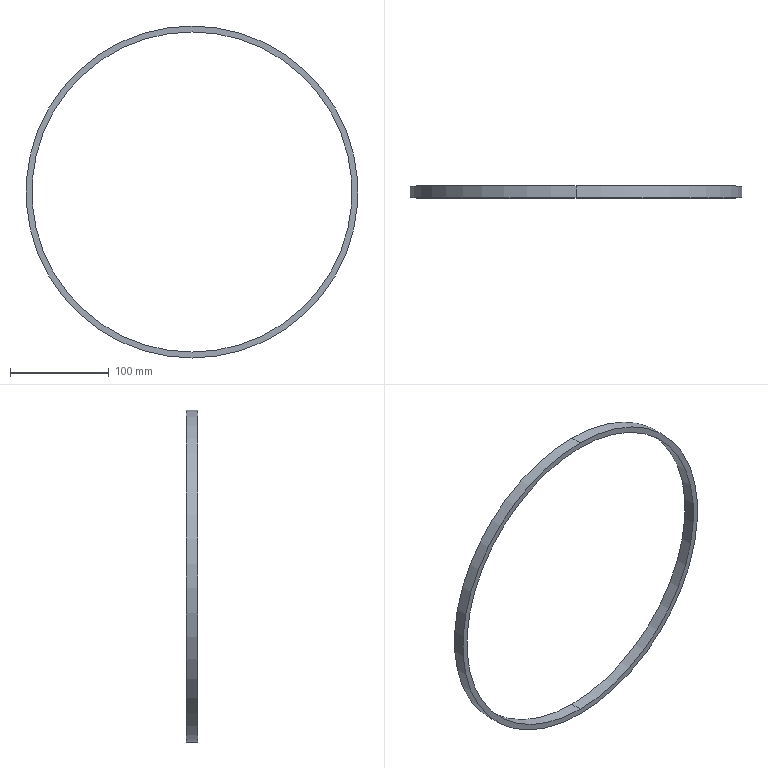Part | SolidWorks | features BaseBody 1, Scale 1 | 1 solid | 6 faces | box 336 x 12 x 336 mm | volume 74644 mm3 | cylinder 4 | plane 2 | commonest cylinder face diameters 324 x2 336 x2
STEP:
#1=CARTESIAN_POINT('',(0.,11.,-168.));
#2=VERTEX_POINT('',#1);
#3=CARTESIAN_POINT('',(0.,11.,168.));
#4=VERTEX_POINT('',#3);
#5=CARTESIAN_POINT('',(0.,11.,0.));
#6=DIRECTION('',(0.,-1.,0.));
#7=DIRECTION('',(0.,0.,-1.));
#8=AXIS2_PLACEMENT_3D('',#5,#6,#7);
#9=CIRCLE('',#8,168.);
#10=EDGE_CURVE('',#2,#4,#9,.T.);
#11=ORIENTED_EDGE('',*,*,#10,.T.);
#12=CARTESIAN_POINT('',(0.,-1.,168.));
#13=VERTEX_POINT('',#12);
#14=CARTESIAN_POINT('',(0.,11.,168.));
#15=DIRECTION('',(0.,-1.,0.));
#16=VECTOR('',#15,1000.);
#17=LINE('',#14,#16);
#18=EDGE_CURVE('',#4,#13,#17,.T.);
#19=ORIENTED_EDGE('',*,*,#18,.T.);
#20=CARTESIAN_POINT('',(0.,-1.,-168.));
#21=VERTEX_POINT('',#20);
#22=CARTESIAN_POINT('',(0.,-1.,0.));
#23=DIRECTION('',(0.,1.,0.));
#24=DIRECTION('',(0.,0.,-1.));
#25=AXIS2_PLACEMENT_3D('',#22,#23,#24);
#26=CIRCLE('',#25,168.);
#27=EDGE_CURVE('',#13,#21,#26,.T.);
#28=ORIENTED_EDGE('',*,*,#27,.T.);
#29=CARTESIAN_POINT('',(0.,11.,-168.));
#30=DIRECTION('',(0.,-1.,0.));
#31=VECTOR('',#30,1000.);
#32=LINE('',#29,#31);
#33=EDGE_CURVE('',#2,#21,#32,.T.);
#34=ORIENTED_EDGE('',*,*,#33,.F.);
#35=EDGE_LOOP('',(#11,#19,#28,#34));
#36=FACE_OUTER_BOUND('',#35,.T.);
#37=CARTESIAN_POINT('',(0.,11.,0.));
#38=DIRECTION('',(0.,-1.,0.));
#39=DIRECTION('',(0.,0.,-1.));
#40=AXIS2_PLACEMENT_3D('',#37,#38,#39);
#41=CYLINDRICAL_SURFACE('',#40,168.);
#42=ADVANCED_FACE('',(#36),#41,.T.);
#43=CARTESIAN_POINT('',(0.,11.,162.));
#44=VERTEX_POINT('',#43);
#45=CARTESIAN_POINT('',(0.,11.,-162.));
#46=VERTEX_POINT('',#45);
#47=CARTESIAN_POINT('',(0.,11.,0.));
#48=DIRECTION('',(0.,-1.,0.));
#49=DIRECTION('',(0.,0.,-1.));
#50=AXIS2_PLACEMENT_3D('',#47,#48,#49);
#51=CIRCLE('',#50,162.);
#52=EDGE_CURVE('',#44,#46,#51,.T.);
#53=ORIENTED_EDGE('',*,*,#52,.F.);
#54=CARTESIAN_POINT('',(0.,-1.,162.));
#55=VERTEX_POINT('',#54);
#56=CARTESIAN_POINT('',(0.,11.,162.));
#57=DIRECTION('',(0.,-1.,0.));
#58=VECTOR('',#57,1000.);
#59=LINE('',#56,#58);
#60=EDGE_CURVE('',#44,#55,#59,.T.);
#61=ORIENTED_EDGE('',*,*,#60,.T.);
#62=CARTESIAN_POINT('',(0.,-1.,-162.));
#63=VERTEX_POINT('',#62);
#64=CARTESIAN_POINT('',(0.,-1.,0.));
#65=DIRECTION('',(0.,-1.,0.));
#66=DIRECTION('',(0.,0.,-1.));
#67=AXIS2_PLACEMENT_3D('',#64,#65,#66);
#68=CIRCLE('',#67,162.);
#69=EDGE_CURVE('',#55,#63,#68,.T.);
#70=ORIENTED_EDGE('',*,*,#69,.T.);
#71=CARTESIAN_POINT('',(0.,11.,-162.));
#72=DIRECTION('',(0.,-1.,0.));
#73=VECTOR('',#72,1000.);
#74=LINE('',#71,#73);
#75=EDGE_CURVE('',#46,#63,#74,.T.);
#76=ORIENTED_EDGE('',*,*,#75,.F.);
#77=EDGE_LOOP('',(#53,#61,#70,#76));
#78=FACE_OUTER_BOUND('',#77,.T.);
#79=CARTESIAN_POINT('',(0.,11.,0.));
#80=DIRECTION('',(0.,-1.,0.));
#81=DIRECTION('',(0.,0.,-1.));
#82=AXIS2_PLACEMENT_3D('',#79,#80,#81);
#83=CYLINDRICAL_SURFACE('',#82,162.);
#84=ADVANCED_FACE('',(#78),#83,.F.);
#85=ORIENTED_EDGE('',*,*,#18,.F.);
#86=CARTESIAN_POINT('',(0.,11.,0.));
#87=DIRECTION('',(0.,-1.,0.));
#88=DIRECTION('',(0.,0.,-1.));
#89=AXIS2_PLACEMENT_3D('',#86,#87,#88);
#90=CIRCLE('',#89,168.);
#91=EDGE_CURVE('',#4,#2,#90,.T.);
#92=ORIENTED_EDGE('',*,*,#91,.T.);
#93=ORIENTED_EDGE('',*,*,#33,.T.);
#94=CARTESIAN_POINT('',(0.,-1.,0.));
#95=DIRECTION('',(0.,1.,0.));
#96=DIRECTION('',(0.,0.,-1.));
#97=AXIS2_PLACEMENT_3D('',#94,#95,#96);
#98=CIRCLE('',#97,168.);
#99=EDGE_CURVE('',#21,#13,#98,.T.);
#100=ORIENTED_EDGE('',*,*,#99,.T.);
#101=EDGE_LOOP('',(#85,#92,#93,#100));
#102=FACE_OUTER_BOUND('',#101,.T.);
#103=CARTESIAN_POINT('',(0.,11.,0.));
#104=DIRECTION('',(0.,-1.,0.));
#105=DIRECTION('',(0.,0.,-1.));
#106=AXIS2_PLACEMENT_3D('',#103,#104,#105);
#107=CYLINDRICAL_SURFACE('',#106,168.);
#108=ADVANCED_FACE('',(#102),#107,.T.);
#109=CARTESIAN_POINT('',(0.,-1.,0.));
#110=DIRECTION('',(0.,-1.,0.));
#111=DIRECTION('',(0.,0.,-1.));
#112=AXIS2_PLACEMENT_3D('',#109,#110,#111);
#113=CIRCLE('',#112,162.);
#114=EDGE_CURVE('',#63,#55,#113,.T.);
#115=ORIENTED_EDGE('',*,*,#114,.F.);
#116=ORIENTED_EDGE('',*,*,#69,.F.);
#117=EDGE_LOOP('',(#115,#116));
#118=FACE_BOUND('',#117,.T.);
#119=ORIENTED_EDGE('',*,*,#99,.F.);
#120=ORIENTED_EDGE('',*,*,#27,.F.);
#121=EDGE_LOOP('',(#119,#120));
#122=FACE_OUTER_BOUND('',#121,.T.);
#123=CARTESIAN_POINT('',(0.,-1.,0.));
#124=DIRECTION('',(0.,1.,0.));
#125=DIRECTION('',(0.,0.,1.));
#126=AXIS2_PLACEMENT_3D('',#123,#124,#125);
#127=PLANE('',#126);
#128=ADVANCED_FACE('',(#118,#122),#127,.F.);
#129=CARTESIAN_POINT('',(0.,11.,0.));
#130=DIRECTION('',(0.,-1.,0.));
#131=DIRECTION('',(0.,0.,-1.));
#132=AXIS2_PLACEMENT_3D('',#129,#130,#131);
#133=CIRCLE('',#132,162.);
#134=EDGE_CURVE('',#46,#44,#133,.T.);
#135=ORIENTED_EDGE('',*,*,#134,.T.);
#136=ORIENTED_EDGE('',*,*,#52,.T.);
#137=EDGE_LOOP('',(#135,#136));
#138=FACE_BOUND('',#137,.T.);
#139=ORIENTED_EDGE('',*,*,#10,.F.);
#140=ORIENTED_EDGE('',*,*,#91,.F.);
#141=EDGE_LOOP('',(#139,#140));
#142=FACE_OUTER_BOUND('',#141,.T.);
#143=CARTESIAN_POINT('',(0.,11.,0.));
#144=DIRECTION('',(0.,1.,0.));
#145=DIRECTION('',(0.,0.,1.));
#146=AXIS2_PLACEMENT_3D('',#143,#144,#145);
#147=PLANE('',#146);
#148=ADVANCED_FACE('',(#138,#142),#147,.T.);
#149=ORIENTED_EDGE('',*,*,#60,.F.);
#150=ORIENTED_EDGE('',*,*,#134,.F.);
#151=ORIENTED_EDGE('',*,*,#75,.T.);
#152=ORIENTED_EDGE('',*,*,#114,.T.);
#153=EDGE_LOOP('',(#149,#150,#151,#152));
#154=FACE_OUTER_BOUND('',#153,.T.);
#155=CARTESIAN_POINT('',(0.,11.,0.));
#156=DIRECTION('',(0.,-1.,0.));
#157=DIRECTION('',(0.,0.,-1.));
#158=AXIS2_PLACEMENT_3D('',#155,#156,#157);
#159=CYLINDRICAL_SURFACE('',#158,162.);
#160=ADVANCED_FACE('',(#154),#159,.F.);
#161=CLOSED_SHELL('',(#42,#84,#108,#128,#148,#160));
#162=MANIFOLD_SOLID_BREP('',#161);
#163=CARTESIAN_POINT('',(0.,0.,0.));
#164=DIRECTION('',(0.,0.,1.));
#165=DIRECTION('',(1.,0.,0.));
#166=AXIS2_PLACEMENT_3D('',#163,#164,#165);
#167=(LENGTH_UNIT()NAMED_UNIT(*)SI_UNIT(.MILLI.,.METRE.));
#168=UNCERTAINTY_MEASURE_WITH_UNIT(LENGTH_MEASURE(0.00001),#167,'','');
#169=(NAMED_UNIT(*)PLANE_ANGLE_UNIT()SI_UNIT($,.RADIAN.));
#170=(NAMED_UNIT(*)SI_UNIT($,.STERADIAN.)SOLID_ANGLE_UNIT());
#171=(GEOMETRIC_REPRESENTATION_CONTEXT(3)GLOBAL_UNCERTAINTY_ASSIGNED_CONTEXT((#168))GLOBAL_UNIT_ASSIGNED_CONTEXT((#167,#169,#170))REPRESENTATION_CONTEXT('',''));
#172=ADVANCED_BREP_SHAPE_REPRESENTATION('',(#162,#166),#171);